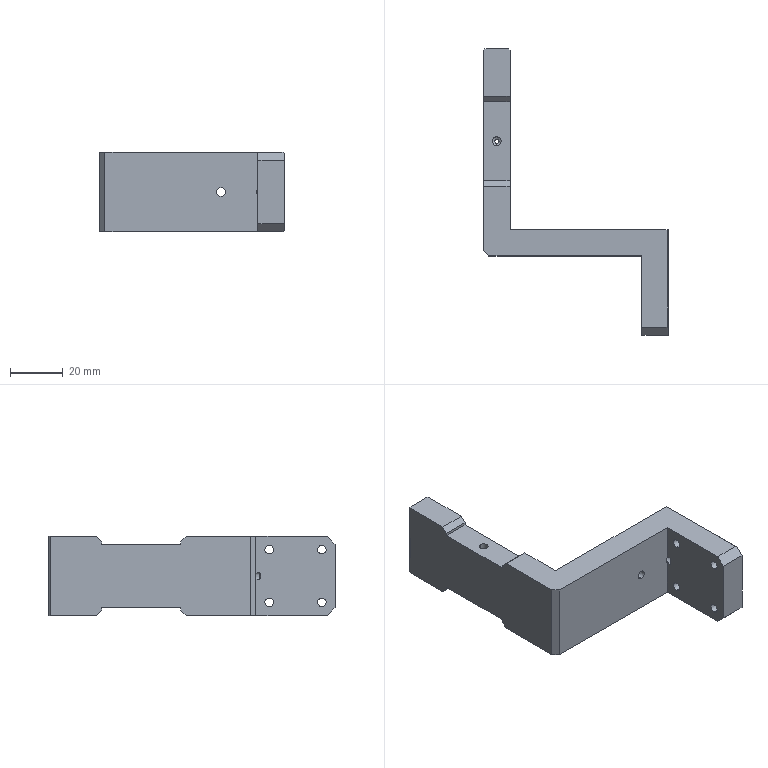Part | SolidWorks | features Chamfer 5, HoleWzd 4, ICE 4, Extrusion 1, MirrorPattern 1 | 1 solid | 62 faces | box 70 x 108.5 x 30 mm | volume 47415 mm3 | plane 30 | cylinder 22 | cone 10 | commonest cylinder face diameters 3.3 x20 5 x2